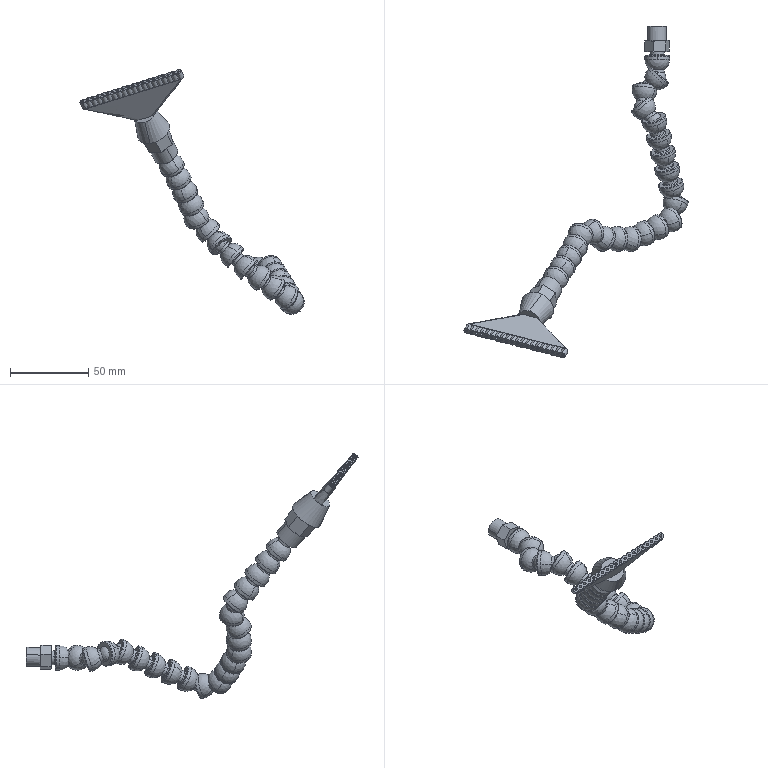Part | SolidWorks | features BaseBody 25, Blend 2, ICE 2 | 23 solids | 633 faces | box 142.999 x 211.658 x 156.105 mm | volume 39289 mm3 | cylinder 244 | sphere 136 | plane 113 | cone 92 | torus 44 | spline 4 | commonest cylinder face diameters 4 x60 7 x46 9 x46 15.811 x44 1.5 x40 16 x4